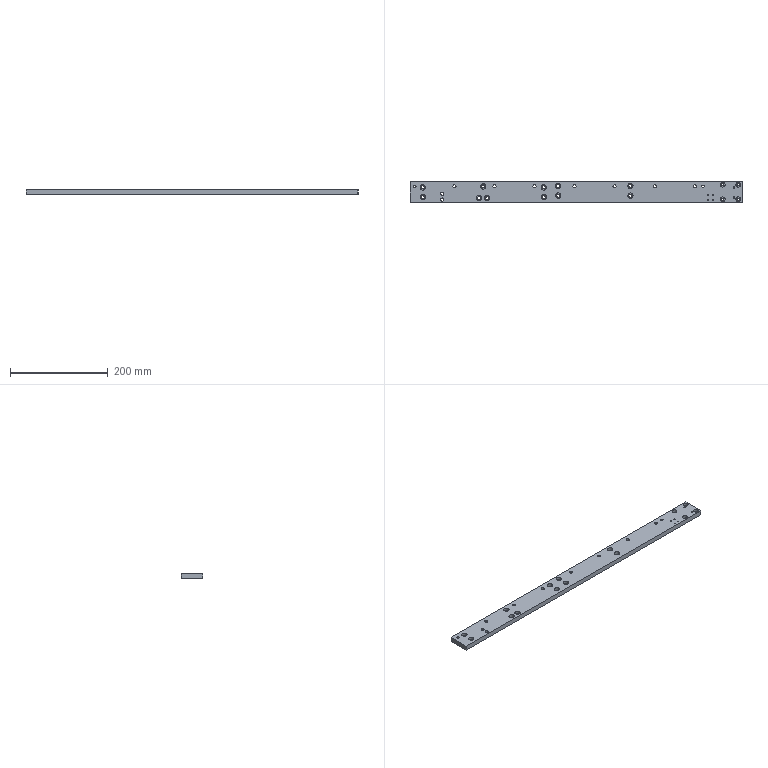Part | SolidWorks | features HoleWzd 10, Chamfer 2, Cut 1, Extrusion 1, LPattern 1 | 1 solid | 154 faces | box 680 x 45 x 10 mm | volume 288393 mm3 | cylinder 112 | plane 34 | cone 8 | commonest cylinder face diameters 11 x40 6.5 x20 6.6 x20 2.5 x8 5.3 x8 10 x8